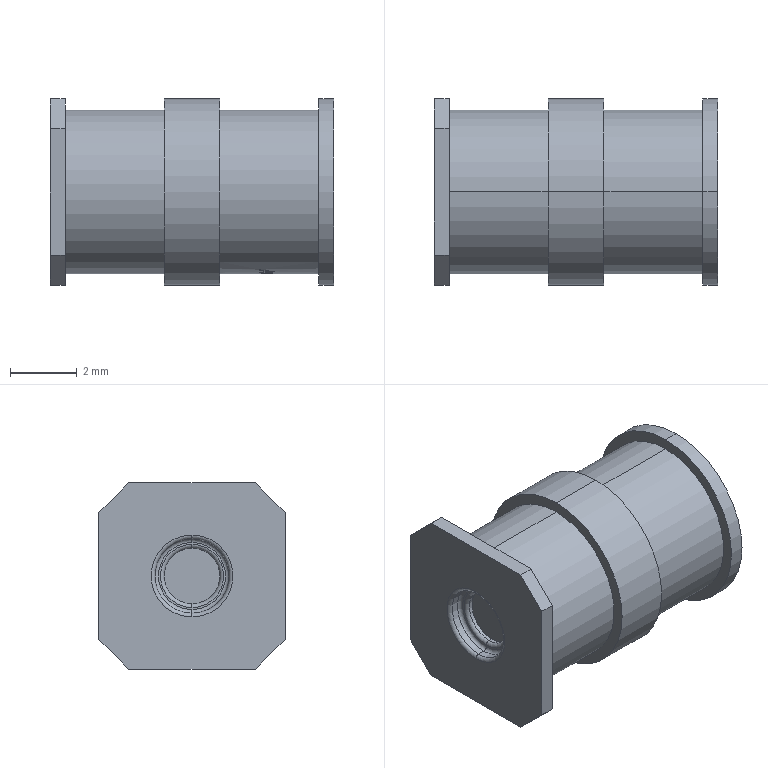Part | NX | features BREP 1 | 1 solid | 93 faces | box 8.512 x 5.6 x 5.6 mm | volume 176.686 mm3 | plane 54 | cylinder 19 | spline 14 | torus 6 | commonest cylinder face diameters 4.928 x6 4.926 x5 5.6 x4 1.68 x2 2.24 x2